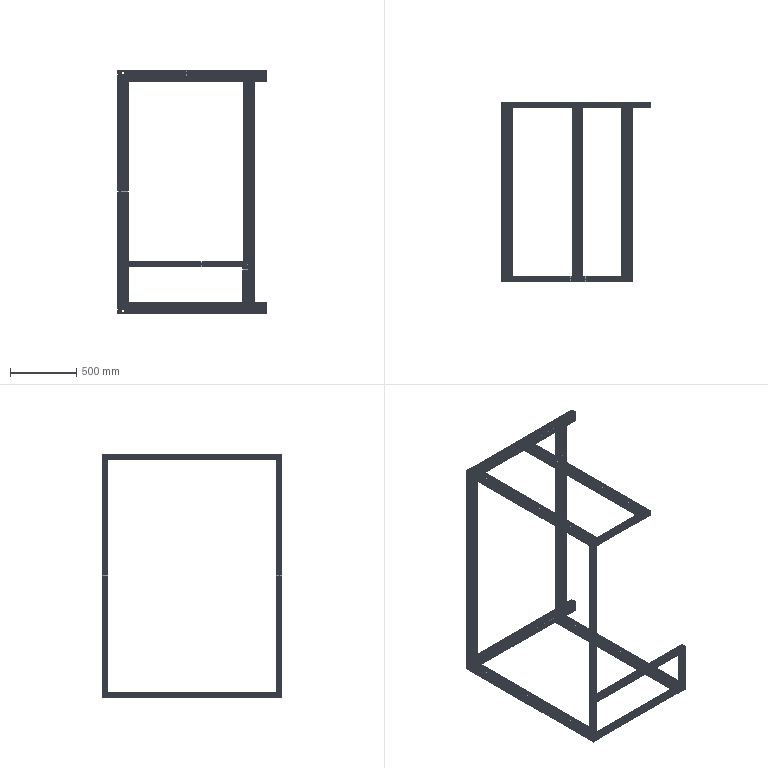Part | NX | features BREP 13 | 13 solids | 3854 faces | volume 16463495 mm3 | cylinder 1951 | plane 1903 | commonest cylinder face diameters 1 x746 0.4 x627 4 x190 6 x104 5 x84 6.8 x64